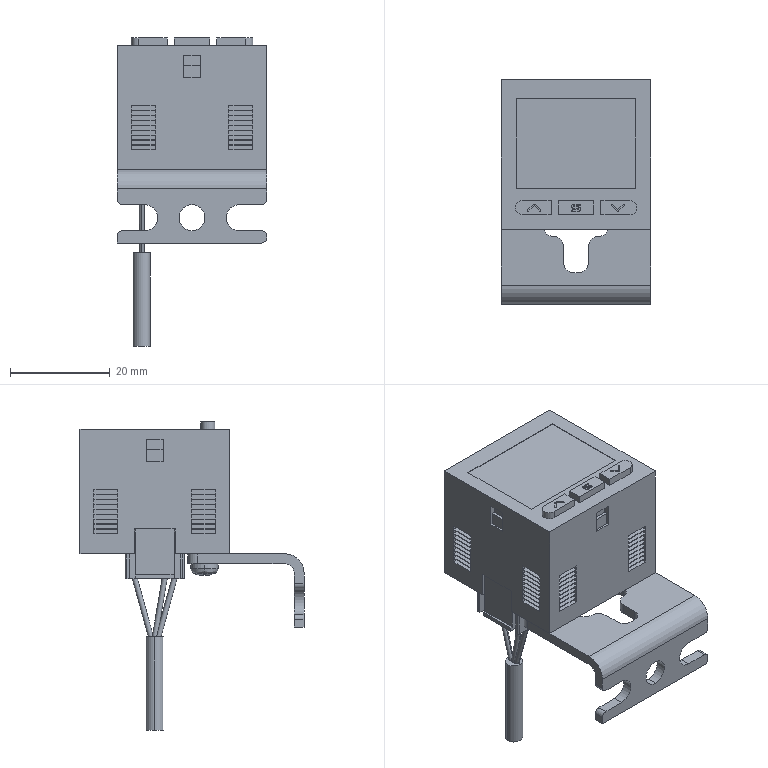Part | SolidWorks | features BaseBody 3 | 3 solids | 704 faces | box 30 x 45 x 61.9 mm | volume 24324 mm3 | plane 577 | cylinder 97 | cone 24 | spline 6 | commonest cylinder face diameters 2 x13 0.3 x12 1.6 x8 2.459 x8 1 x6 4 x6